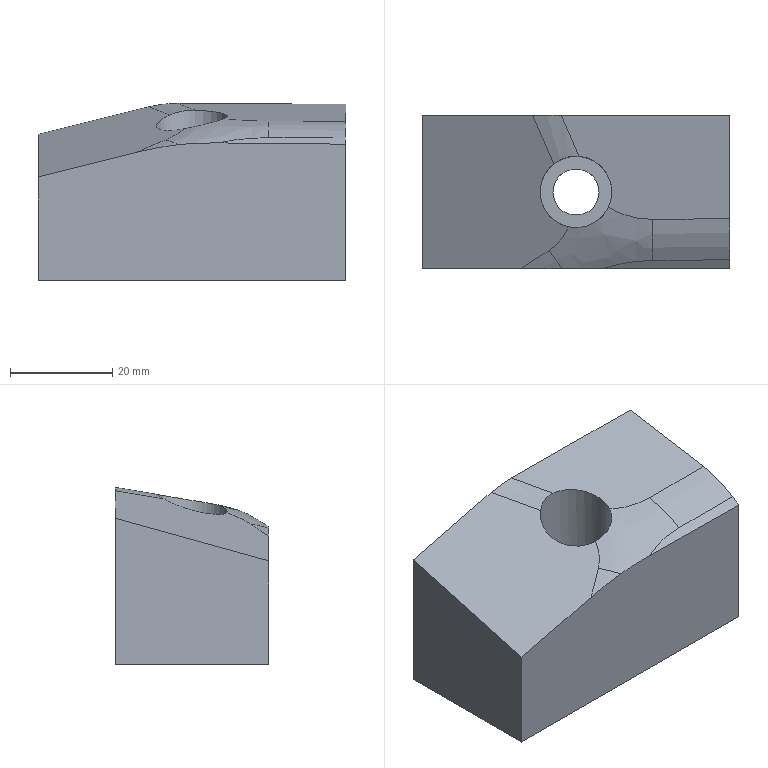Part | NX | features solid 2 | 1 solid | 15 faces | box 60 x 30.012 x 34.633 mm | volume 49926 mm3 | spline 7 | plane 6 | cylinder 2 | commonest cylinder face diameters 9 x1 14 x1
STEP:
#1=CARTESIAN_POINT('',(640.075,-255.006,46.91));
#2=VERTEX_POINT('',#1);
#3=CARTESIAN_POINT('',(665.,-255.,46.666));
#4=VERTEX_POINT('',#3);
#5=CARTESIAN_POINT('',(603.284,-255.,47.28));
#6=DIRECTION('',(1.,0.,-0.009937));
#7=VECTOR('',#6,1000.);
#8=LINE('',#5,#7);
#9=EDGE_CURVE('',#2,#4,#8,.T.);
#10=ORIENTED_EDGE('',*,*,#9,.F.);
#11=CARTESIAN_POINT('',(632.351,-255.,46.58));
#12=VERTEX_POINT('',#11);
#13=CARTESIAN_POINT('',(640.063,-255.,46.914));
#14=CARTESIAN_POINT('',(637.484,-255.,46.936));
#15=CARTESIAN_POINT('',(634.908,-255.,46.878));
#16=CARTESIAN_POINT('',(632.35,-255.,46.58));
#17=B_SPLINE_CURVE_WITH_KNOTS('',3,(#13,#14,#15,#16),.UNSPECIFIED.,.F.,.F.,(4,4),(0.007821,0.01556),.UNSPECIFIED.);
#18=EDGE_CURVE('',#2,#12,#17,.T.);
#19=ORIENTED_EDGE('',*,*,#18,.T.);
#20=CARTESIAN_POINT('',(624.182,-255.,45.074));
#21=VERTEX_POINT('',#20);
#22=CARTESIAN_POINT('',(624.182,-255.,45.074));
#23=CARTESIAN_POINT('',(626.871,-255.,45.746));
#24=CARTESIAN_POINT('',(629.597,-255.,46.262));
#25=CARTESIAN_POINT('',(632.351,-255.,46.58));
#26=B_SPLINE_CURVE_WITH_KNOTS('',3,(#22,#23,#24,#25),.UNSPECIFIED.,.F.,.F.,(4,4),(0.,0.008311),.UNSPECIFIED.);
#27=EDGE_CURVE('',#21,#12,#26,.T.);
#28=ORIENTED_EDGE('',*,*,#27,.F.);
#29=CARTESIAN_POINT('',(605.,-255.,40.28));
#30=VERTEX_POINT('',#29);
#31=CARTESIAN_POINT('',(605.,-255.,40.28));
#32=CARTESIAN_POINT('',(611.394,-255.,41.878));
#33=CARTESIAN_POINT('',(617.788,-255.,43.476));
#34=CARTESIAN_POINT('',(624.182,-255.,45.074));
#35=B_SPLINE_CURVE_WITH_KNOTS('',3,(#31,#32,#33,#34),.UNSPECIFIED.,.F.,.F.,(4,4),(0.,0.01977),.UNSPECIFIED.);
#36=EDGE_CURVE('',#30,#21,#35,.T.);
#37=ORIENTED_EDGE('',*,*,#36,.F.);
#38=CARTESIAN_POINT('',(605.,-255.,20.));
#39=VERTEX_POINT('',#38);
#40=CARTESIAN_POINT('',(605.,-255.,220.));
#41=DIRECTION('',(0.,0.,-1.));
#42=VECTOR('',#41,1000.);
#43=LINE('',#40,#42);
#44=EDGE_CURVE('',#30,#39,#43,.T.);
#45=ORIENTED_EDGE('',*,*,#44,.T.);
#46=CARTESIAN_POINT('',(665.,-255.,20.));
#47=VERTEX_POINT('',#46);
#48=CARTESIAN_POINT('',(605.,-255.,20.));
#49=DIRECTION('',(1.,0.,0.));
#50=VECTOR('',#49,1000.);
#51=LINE('',#48,#50);
#52=EDGE_CURVE('',#39,#47,#51,.T.);
#53=ORIENTED_EDGE('',*,*,#52,.T.);
#54=CARTESIAN_POINT('',(665.,-255.,220.));
#55=DIRECTION('',(0.,0.,1.));
#56=VECTOR('',#55,1000.);
#57=LINE('',#54,#56);
#58=EDGE_CURVE('',#4,#47,#57,.F.);
#59=ORIENTED_EDGE('',*,*,#58,.F.);
#60=EDGE_LOOP('',(#10,#19,#28,#37,#45,#53,#59));
#61=FACE_BOUND('',#60,.T.);
#62=CARTESIAN_POINT('',(605.,-255.,220.));
#63=DIRECTION('',(0.,1.,0.));
#64=DIRECTION('',(0.,0.,-1.));
#65=AXIS2_PLACEMENT_3D('',#62,#63,#64);
#66=PLANE('',#65);
#67=ADVANCED_FACE('',(#61),#66,.F.);
#68=CARTESIAN_POINT('',(639.5,-240.,20.));
#69=VERTEX_POINT('',#68);
#70=CARTESIAN_POINT('',(635.,-240.,20.));
#71=DIRECTION('',(0.,0.,1.));
#72=DIRECTION('',(1.,0.,0.));
#73=AXIS2_PLACEMENT_3D('',#70,#71,#72);
#74=CIRCLE('',#73,4.5);
#75=EDGE_CURVE('',#69,#69,#74,.F.);
#76=ORIENTED_EDGE('',*,*,#75,.F.);
#77=EDGE_LOOP('',(#76));
#78=FACE_BOUND('',#77,.T.);
#79=ORIENTED_EDGE('',*,*,#52,.F.);
#80=CARTESIAN_POINT('',(605.,-225.,20.));
#81=VERTEX_POINT('',#80);
#82=CARTESIAN_POINT('',(605.,-255.,20.));
#83=DIRECTION('',(0.,1.,0.));
#84=VECTOR('',#83,1000.);
#85=LINE('',#82,#84);
#86=EDGE_CURVE('',#39,#81,#85,.T.);
#87=ORIENTED_EDGE('',*,*,#86,.T.);
#88=CARTESIAN_POINT('',(665.,-225.,20.));
#89=VERTEX_POINT('',#88);
#90=CARTESIAN_POINT('',(605.,-225.,20.));
#91=DIRECTION('',(1.,0.,0.));
#92=VECTOR('',#91,1000.);
#93=LINE('',#90,#92);
#94=EDGE_CURVE('',#81,#89,#93,.T.);
#95=ORIENTED_EDGE('',*,*,#94,.T.);
#96=CARTESIAN_POINT('',(665.,-255.,20.));
#97=DIRECTION('',(0.,1.,0.));
#98=VECTOR('',#97,1000.);
#99=LINE('',#96,#98);
#100=EDGE_CURVE('',#47,#89,#99,.T.);
#101=ORIENTED_EDGE('',*,*,#100,.F.);
#102=EDGE_LOOP('',(#79,#87,#95,#101));
#103=FACE_BOUND('',#102,.T.);
#104=CARTESIAN_POINT('',(605.,-255.,20.));
#105=DIRECTION('',(0.,0.,1.));
#106=DIRECTION('',(0.,1.,0.));
#107=AXIS2_PLACEMENT_3D('',#104,#105,#106);
#108=PLANE('',#107);
#109=ADVANCED_FACE('',(#78,#103),#108,.F.);
#110=CARTESIAN_POINT('',(665.,-225.,54.456));
#111=VERTEX_POINT('',#110);
#112=CARTESIAN_POINT('',(665.,-225.,220.));
#113=DIRECTION('',(0.,0.,1.));
#114=VECTOR('',#113,1000.);
#115=LINE('',#112,#114);
#116=EDGE_CURVE('',#111,#89,#115,.F.);
#117=ORIENTED_EDGE('',*,*,#116,.F.);
#118=CARTESIAN_POINT('',(665.,-245.237,51.089));
#119=VERTEX_POINT('',#118);
#120=CARTESIAN_POINT('',(665.,-227.393,54.058));
#121=DIRECTION('',(0.,0.9864,0.1641));
#122=VECTOR('',#121,1000.);
#123=LINE('',#120,#122);
#124=EDGE_CURVE('',#111,#119,#123,.F.);
#125=ORIENTED_EDGE('',*,*,#124,.T.);
#126=CARTESIAN_POINT('',(665.,-253.26,47.859));
#127=VERTEX_POINT('',#126);
#128=CARTESIAN_POINT('',(665.,-245.237,51.089));
#129=CARTESIAN_POINT('',(665.,-248.111,50.611));
#130=CARTESIAN_POINT('',(665.,-250.857,49.505));
#131=CARTESIAN_POINT('',(665.,-253.26,47.859));
#132=B_SPLINE_CURVE_WITH_KNOTS('',3,(#128,#129,#130,#131),.UNSPECIFIED.,.F.,.F.,(4,4),(0.00005182,0.008777),.UNSPECIFIED.);
#133=EDGE_CURVE('',#119,#127,#132,.T.);
#134=ORIENTED_EDGE('',*,*,#133,.T.);
#135=CARTESIAN_POINT('',(665.,-174.178,102.045));
#136=DIRECTION('',(0.,0.8249,0.5652));
#137=VECTOR('',#136,1000.);
#138=LINE('',#135,#137);
#139=EDGE_CURVE('',#127,#4,#138,.F.);
#140=ORIENTED_EDGE('',*,*,#139,.T.);
#141=ORIENTED_EDGE('',*,*,#58,.T.);
#142=ORIENTED_EDGE('',*,*,#100,.T.);
#143=EDGE_LOOP('',(#117,#125,#134,#140,#141,#142));
#144=FACE_BOUND('',#143,.T.);
#145=CARTESIAN_POINT('',(665.,-255.,220.));
#146=DIRECTION('',(-1.,0.,0.));
#147=DIRECTION('',(0.,0.,1.));
#148=AXIS2_PLACEMENT_3D('',#145,#146,#147);
#149=PLANE('',#148);
#150=ADVANCED_FACE('',(#144),#149,.F.);
#151=CARTESIAN_POINT('',(632.136,-225.,54.632));
#152=VERTEX_POINT('',#151);
#153=CARTESIAN_POINT('',(604.112,-225.,54.783));
#154=DIRECTION('',(1.,0.,-0.005377));
#155=VECTOR('',#154,1000.);
#156=LINE('',#153,#155);
#157=EDGE_CURVE('',#111,#152,#156,.F.);
#158=ORIENTED_EDGE('',*,*,#157,.F.);
#159=ORIENTED_EDGE('',*,*,#116,.T.);
#160=ORIENTED_EDGE('',*,*,#94,.F.);
#161=CARTESIAN_POINT('',(605.,-225.,48.586));
#162=VERTEX_POINT('',#161);
#163=CARTESIAN_POINT('',(605.,-225.,220.));
#164=DIRECTION('',(0.,0.,-1.));
#165=VECTOR('',#164,1000.);
#166=LINE('',#163,#165);
#167=EDGE_CURVE('',#162,#81,#166,.T.);
#168=ORIENTED_EDGE('',*,*,#167,.F.);
#169=CARTESIAN_POINT('',(626.522,-225.,53.964));
#170=VERTEX_POINT('',#169);
#171=CARTESIAN_POINT('',(626.522,-225.,53.964));
#172=CARTESIAN_POINT('',(619.348,-225.,52.172));
#173=CARTESIAN_POINT('',(612.174,-225.,50.379));
#174=CARTESIAN_POINT('',(605.,-225.,48.586));
#175=B_SPLINE_CURVE_WITH_KNOTS('',3,(#171,#172,#173,#174),.UNSPECIFIED.,.F.,.F.,(4,4),(0.007848,0.03003),.UNSPECIFIED.);
#176=EDGE_CURVE('',#170,#162,#175,.T.);
#177=ORIENTED_EDGE('',*,*,#176,.F.);
#178=CARTESIAN_POINT('',(632.136,-225.,54.632));
#179=CARTESIAN_POINT('',(630.245,-225.,54.643));
#180=CARTESIAN_POINT('',(628.356,-225.,54.423));
#181=CARTESIAN_POINT('',(626.522,-225.,53.964));
#182=B_SPLINE_CURVE_WITH_KNOTS('',3,(#178,#179,#180,#181),.UNSPECIFIED.,.F.,.F.,(4,4),(0.,0.005662),.UNSPECIFIED.);
#183=EDGE_CURVE('',#152,#170,#182,.T.);
#184=ORIENTED_EDGE('',*,*,#183,.F.);
#185=EDGE_LOOP('',(#158,#159,#160,#168,#177,#184));
#186=FACE_BOUND('',#185,.T.);
#187=CARTESIAN_POINT('',(605.,-225.,220.));
#188=DIRECTION('',(0.,1.,0.));
#189=DIRECTION('',(0.,0.,-1.));
#190=AXIS2_PLACEMENT_3D('',#187,#188,#189);
#191=PLANE('',#190);
#192=ADVANCED_FACE('',(#186),#191,.T.);
#193=CARTESIAN_POINT('',(605.,-208.786,53.075));
#194=DIRECTION('',(0.,0.9637,0.2668));
#195=VECTOR('',#194,1000.);
#196=LINE('',#193,#195);
#197=EDGE_CURVE('',#162,#30,#196,.F.);
#198=ORIENTED_EDGE('',*,*,#197,.F.);
#199=ORIENTED_EDGE('',*,*,#167,.T.);
#200=ORIENTED_EDGE('',*,*,#86,.F.);
#201=ORIENTED_EDGE('',*,*,#44,.F.);
#202=EDGE_LOOP('',(#198,#199,#200,#201));
#203=FACE_BOUND('',#202,.T.);
#204=CARTESIAN_POINT('',(605.,-255.,220.));
#205=DIRECTION('',(-1.,0.,0.));
#206=DIRECTION('',(0.,0.,1.));
#207=AXIS2_PLACEMENT_3D('',#204,#205,#206);
#208=PLANE('',#207);
#209=ADVANCED_FACE('',(#203),#208,.T.);
#210=ORIENTED_EDGE('',*,*,#133,.F.);
#211=CARTESIAN_POINT('',(649.965,-245.37,51.148));
#212=VERTEX_POINT('',#211);
#213=CARTESIAN_POINT('',(665.,-245.237,51.089));
#214=CARTESIAN_POINT('',(659.988,-245.281,51.108));
#215=CARTESIAN_POINT('',(654.977,-245.326,51.128));
#216=CARTESIAN_POINT('',(649.965,-245.37,51.148));
#217=B_SPLINE_CURVE_WITH_KNOTS('',3,(#213,#214,#215,#216),.UNSPECIFIED.,.F.,.F.,(4,4),(0.8008,1.),.UNSPECIFIED.);
#218=EDGE_CURVE('',#212,#119,#217,.F.);
#219=ORIENTED_EDGE('',*,*,#218,.F.);
#220=CARTESIAN_POINT('',(650.023,-253.392,47.917));
#221=VERTEX_POINT('',#220);
#222=CARTESIAN_POINT('',(649.965,-245.37,51.148));
#223=CARTESIAN_POINT('',(649.988,-248.214,50.674));
#224=CARTESIAN_POINT('',(650.008,-251.014,49.546));
#225=CARTESIAN_POINT('',(650.023,-253.392,47.917));
#226=B_SPLINE_CURVE_WITH_KNOTS('',3,(#222,#223,#224,#225),.UNSPECIFIED.,.F.,.F.,(4,4),(0.,1.),.UNSPECIFIED.);
#227=EDGE_CURVE('',#212,#221,#226,.T.);
#228=ORIENTED_EDGE('',*,*,#227,.T.);
#229=CARTESIAN_POINT('',(650.023,-253.392,47.917));
#230=CARTESIAN_POINT('',(655.015,-253.348,47.898));
#231=CARTESIAN_POINT('',(660.008,-253.304,47.878));
#232=CARTESIAN_POINT('',(665.,-253.26,47.859));
#233=B_SPLINE_CURVE_WITH_KNOTS('',3,(#229,#230,#231,#232),.UNSPECIFIED.,.F.,.F.,(4,4),(0.,0.2001),.UNSPECIFIED.);
#234=EDGE_CURVE('',#221,#127,#233,.T.);
#235=ORIENTED_EDGE('',*,*,#234,.T.);
#236=EDGE_LOOP('',(#210,#219,#228,#235));
#237=FACE_BOUND('',#236,.T.);
#238=CARTESIAN_POINT('',(665.148,-253.259,47.858));
#239=CARTESIAN_POINT('',(650.023,-253.392,47.917));
#240=CARTESIAN_POINT('',(665.133,-250.843,49.514));
#241=CARTESIAN_POINT('',(650.008,-250.976,49.573));
#242=CARTESIAN_POINT('',(665.114,-248.126,50.608));
#243=CARTESIAN_POINT('',(649.988,-248.259,50.667));
#244=CARTESIAN_POINT('',(665.09,-245.237,51.088));
#245=CARTESIAN_POINT('',(649.965,-245.37,51.148));
#246=(BOUNDED_SURFACE()B_SPLINE_SURFACE(3,1,((#238,#239),(#240,#241),(#242,#243),(#244,#245)),.CYLINDRICAL_SURF.,.F.,.F.,.F.)B_SPLINE_SURFACE_WITH_KNOTS((4,4),(2,2),(0.,0.994),(0.8008,1.),.PIECEWISE_BEZIER_KNOTS.)GEOMETRIC_REPRESENTATION_ITEM()RATIONAL_B_SPLINE_SURFACE(((1.,1.),(0.9841,0.9841),(0.984,0.984),(0.9997,0.9997)))REPRESENTATION_ITEM('')SURFACE());
#247=ADVANCED_FACE('',(#237),#246,.T.);
#248=CARTESIAN_POINT('',(633.516,-246.841,49.666));
#249=VERTEX_POINT('',#248);
#250=CARTESIAN_POINT('',(629.735,-251.466,47.441));
#251=VERTEX_POINT('',#250);
#252=CARTESIAN_POINT('',(629.735,-251.466,47.44));
#253=CARTESIAN_POINT('',(630.556,-250.944,47.79));
#254=CARTESIAN_POINT('',(632.008,-249.638,48.515));
#255=CARTESIAN_POINT('',(633.064,-247.909,49.257));
#256=CARTESIAN_POINT('',(633.516,-246.841,49.666));
#257=B_SPLINE_CURVE_WITH_KNOTS('',3,(#252,#253,#254,#255,#256),.UNSPECIFIED.,.F.,.F.,(4,1,4),(0.,0.2636,0.5272),.UNSPECIFIED.);
#258=EDGE_CURVE('',#249,#251,#257,.F.);
#259=ORIENTED_EDGE('',*,*,#258,.F.);
#260=CARTESIAN_POINT('',(630.643,-234.522,52.358));
#261=VERTEX_POINT('',#260);
#262=CARTESIAN_POINT('',(633.516,-246.841,49.666));
#263=CARTESIAN_POINT('',(632.219,-246.56,49.42));
#264=CARTESIAN_POINT('',(629.723,-245.204,49.171));
#265=CARTESIAN_POINT('',(627.761,-241.464,49.716));
#266=CARTESIAN_POINT('',(628.102,-237.439,50.916));
#267=CARTESIAN_POINT('',(629.652,-235.309,51.892));
#268=CARTESIAN_POINT('',(630.643,-234.522,52.358));
#269=B_SPLINE_CURVE_WITH_KNOTS('',3,(#262,#263,#264,#265,#266,#267,#268),.UNSPECIFIED.,.F.,.F.,(4,1,1,1,4),(0.001037,0.005085,0.009132,0.01318,0.01723),.UNSPECIFIED.);
#270=EDGE_CURVE('',#249,#261,#269,.T.);
#271=ORIENTED_EDGE('',*,*,#270,.T.);
#272=CARTESIAN_POINT('',(630.643,-234.522,52.358));
#273=CARTESIAN_POINT('',(629.269,-231.348,52.894));
#274=CARTESIAN_POINT('',(627.895,-228.174,53.429));
#275=CARTESIAN_POINT('',(626.522,-225.,53.964));
#276=B_SPLINE_CURVE_WITH_KNOTS('',3,(#272,#273,#274,#275),.UNSPECIFIED.,.F.,.F.,(4,4),(0.06874,0.1608),.UNSPECIFIED.);
#277=EDGE_CURVE('',#170,#261,#276,.F.);
#278=ORIENTED_EDGE('',*,*,#277,.F.);
#279=ORIENTED_EDGE('',*,*,#176,.T.);
#280=ORIENTED_EDGE('',*,*,#197,.T.);
#281=ORIENTED_EDGE('',*,*,#36,.T.);
#282=CARTESIAN_POINT('',(624.182,-255.,45.074));
#283=CARTESIAN_POINT('',(626.033,-253.822,45.863));
#284=CARTESIAN_POINT('',(627.884,-252.644,46.652));
#285=CARTESIAN_POINT('',(629.735,-251.466,47.44));
#286=B_SPLINE_CURVE_WITH_KNOTS('',3,(#282,#283,#284,#285),.UNSPECIFIED.,.F.,.F.,(4,4),(0.868,1.),.UNSPECIFIED.);
#287=EDGE_CURVE('',#251,#21,#286,.F.);
#288=ORIENTED_EDGE('',*,*,#287,.F.);
#289=EDGE_LOOP('',(#259,#271,#278,#279,#280,#281,#288));
#290=FACE_BOUND('',#289,.T.);
#291=CARTESIAN_POINT('',(633.196,-225.095,55.606));
#292=CARTESIAN_POINT('',(633.904,-256.4,47.116));
#293=CARTESIAN_POINT('',(604.124,-223.874,48.679));
#294=CARTESIAN_POINT('',(604.832,-255.178,40.189));
#295=B_SPLINE_SURFACE_WITH_KNOTS('',1,1,((#291,#292),(#293,#294)),.PLANE_SURF.,.F.,.F.,.F.,(2,2),(2,2),(0.01963,0.6254),(0.6059,0.8264),.PIECEWISE_BEZIER_KNOTS.);
#296=ADVANCED_FACE('',(#290),#295,.T.);
#297=ORIENTED_EDGE('',*,*,#287,.T.);
#298=ORIENTED_EDGE('',*,*,#27,.T.);
#299=CARTESIAN_POINT('',(632.351,-255.,46.58));
#300=CARTESIAN_POINT('',(631.451,-253.882,47.021));
#301=CARTESIAN_POINT('',(630.569,-252.689,47.31));
#302=CARTESIAN_POINT('',(629.735,-251.466,47.44));
#303=B_SPLINE_CURVE_WITH_KNOTS('',3,(#299,#300,#301,#302),.UNSPECIFIED.,.F.,.F.,(4,4),(0.4511,1.),.UNSPECIFIED.);
#304=EDGE_CURVE('',#251,#12,#303,.F.);
#305=ORIENTED_EDGE('',*,*,#304,.F.);
#306=EDGE_LOOP('',(#297,#298,#305));
#307=FACE_BOUND('',#306,.T.);
#308=CARTESIAN_POINT('',(632.367,-255.02,46.572));
#309=CARTESIAN_POINT('',(626.78,-258.575,44.192));
#310=CARTESIAN_POINT('',(631.461,-253.896,47.018));
#311=CARTESIAN_POINT('',(625.874,-257.451,44.638));
#312=CARTESIAN_POINT('',(630.58,-252.706,47.308));
#313=CARTESIAN_POINT('',(624.993,-256.261,44.928));
#314=CARTESIAN_POINT('',(629.735,-251.466,47.44));
#315=CARTESIAN_POINT('',(624.148,-255.021,45.06));
#316=(BOUNDED_SURFACE()B_SPLINE_SURFACE(3,1,((#308,#309),(#310,#311),(#312,#313),(#314,#315)),.CYLINDRICAL_SURF.,.F.,.F.,.F.)B_SPLINE_SURFACE_WITH_KNOTS((4,4),(2,2),(0.4511,1.),(0.,0.1192),.PIECEWISE_BEZIER_KNOTS.)GEOMETRIC_REPRESENTATION_ITEM()RATIONAL_B_SPLINE_SURFACE(((0.9896,0.9896),(0.9888,0.9888),(0.9923,0.9923),(1.,1.)))REPRESENTATION_ITEM('')SURFACE());
#317=ADVANCED_FACE('',(#307),#316,.T.);
#318=ORIENTED_EDGE('',*,*,#277,.T.);
#319=CARTESIAN_POINT('',(635.61,-233.027,53.278));
#320=VERTEX_POINT('',#319);
#321=CARTESIAN_POINT('',(630.643,-234.522,52.358));
#322=CARTESIAN_POINT('',(631.98,-233.458,52.987));
#323=CARTESIAN_POINT('',(633.794,-232.868,53.314));
#324=CARTESIAN_POINT('',(635.61,-233.027,53.278));
#325=B_SPLINE_CURVE_WITH_KNOTS('',3,(#321,#322,#323,#324),.UNSPECIFIED.,.F.,.F.,(4,4),(0.,0.005439),.UNSPECIFIED.);
#326=EDGE_CURVE('',#261,#320,#325,.T.);
#327=ORIENTED_EDGE('',*,*,#326,.T.);
#328=CARTESIAN_POINT('',(635.61,-233.027,53.278));
#329=CARTESIAN_POINT('',(634.452,-230.351,53.73));
#330=CARTESIAN_POINT('',(633.294,-227.676,54.181));
#331=CARTESIAN_POINT('',(632.136,-225.,54.632));
#332=B_SPLINE_CURVE_WITH_KNOTS('',3,(#328,#329,#330,#331),.UNSPECIFIED.,.F.,.F.,(4,4),(0.06014,0.1322),.UNSPECIFIED.);
#333=EDGE_CURVE('',#152,#320,#332,.F.);
#334=ORIENTED_EDGE('',*,*,#333,.F.);
#335=ORIENTED_EDGE('',*,*,#183,.T.);
#336=EDGE_LOOP('',(#318,#327,#334,#335));
#337=FACE_BOUND('',#336,.T.);
#338=CARTESIAN_POINT('',(630.846,-234.992,52.279));
#339=CARTESIAN_POINT('',(626.496,-224.94,53.974));
#340=CARTESIAN_POINT('',(632.411,-234.408,52.832));
#341=CARTESIAN_POINT('',(628.061,-224.356,54.527));
#342=CARTESIAN_POINT('',(634.017,-233.769,53.163));
#343=CARTESIAN_POINT('',(629.667,-223.717,54.859));
#344=CARTESIAN_POINT('',(635.635,-233.086,53.268));
#345=CARTESIAN_POINT('',(631.285,-223.035,54.964));
#346=(BOUNDED_SURFACE()B_SPLINE_SURFACE(3,1,((#338,#339),(#340,#341),(#342,#343),(#344,#345)),.CYLINDRICAL_SURF.,.F.,.F.,.F.)B_SPLINE_SURFACE_WITH_KNOTS((4,4),(2,2),(0.005982,1.),(0.05925,0.1489),.PIECEWISE_BEZIER_KNOTS.)GEOMETRIC_REPRESENTATION_ITEM()RATIONAL_B_SPLINE_SURFACE(((0.9999,0.9999),(0.9942,0.9942),(0.9942,0.9942),(1.,1.)))REPRESENTATION_ITEM('')SURFACE());
#347=ADVANCED_FACE('',(#337),#346,.T.);
#348=CARTESIAN_POINT('',(641.335,-242.979,51.592));
#349=VERTEX_POINT('',#348);
#350=CARTESIAN_POINT('',(633.516,-246.841,49.666));
#351=CARTESIAN_POINT('',(635.064,-247.177,49.957));
#352=CARTESIAN_POINT('',(638.33,-246.761,50.67));
#353=CARTESIAN_POINT('',(640.659,-244.415,51.355));
#354=CARTESIAN_POINT('',(641.335,-242.979,51.592));
#355=B_SPLINE_CURVE_WITH_KNOTS('',3,(#350,#351,#352,#353,#354),.UNSPECIFIED.,.F.,.F.,(4,1,4),(0.008355,0.01314,0.01793),.UNSPECIFIED.);
#356=EDGE_CURVE('',#249,#349,#355,.T.);
#357=ORIENTED_EDGE('',*,*,#356,.F.);
#358=ORIENTED_EDGE('',*,*,#258,.T.);
#359=ORIENTED_EDGE('',*,*,#304,.T.);
#360=ORIENTED_EDGE('',*,*,#18,.F.);
#361=CARTESIAN_POINT('',(640.088,-255.012,46.906));
#362=CARTESIAN_POINT('',(640.889,-254.747,47.079));
#363=CARTESIAN_POINT('',(642.562,-254.276,47.386));
#364=CARTESIAN_POINT('',(645.818,-253.621,47.801));
#365=CARTESIAN_POINT('',(648.333,-253.407,47.924));
#366=CARTESIAN_POINT('',(650.023,-253.392,47.918));
#367=B_SPLINE_CURVE_WITH_KNOTS('',3,(#361,#362,#363,#364,#365,#366),.UNSPECIFIED.,.F.,.F.,(4,1,1,4),(0.3883,0.5412,0.6942,1.),.UNSPECIFIED.);
#368=EDGE_CURVE('',#221,#2,#367,.F.);
#369=ORIENTED_EDGE('',*,*,#368,.F.);
#370=ORIENTED_EDGE('',*,*,#227,.F.);
#371=CARTESIAN_POINT('',(649.965,-245.37,51.148));
#372=CARTESIAN_POINT('',(648.459,-245.383,51.154));
#373=CARTESIAN_POINT('',(646.227,-245.087,51.214));
#374=CARTESIAN_POINT('',(643.503,-244.18,51.381));
#375=CARTESIAN_POINT('',(641.962,-243.398,51.519));
#376=CARTESIAN_POINT('',(641.335,-242.979,51.592));
#377=B_SPLINE_CURVE_WITH_KNOTS('',3,(#371,#372,#373,#374,#375,#376),.UNSPECIFIED.,.F.,.F.,(4,1,1,4),(0.,0.3269,0.4903,0.6537),.UNSPECIFIED.);
#378=EDGE_CURVE('',#349,#212,#377,.F.);
#379=ORIENTED_EDGE('',*,*,#378,.F.);
#380=EDGE_LOOP('',(#357,#358,#359,#360,#369,#370,#379));
#381=FACE_BOUND('',#380,.T.);
#382=CARTESIAN_POINT('',(631.012,-257.176,45.293));
#383=CARTESIAN_POINT('',(630.414,-254.95,46.483));
#384=CARTESIAN_POINT('',(629.832,-252.628,47.428));
#385=CARTESIAN_POINT('',(629.287,-250.072,47.772));
#386=CARTESIAN_POINT('',(628.747,-247.484,48.036));
#387=CARTESIAN_POINT('',(628.199,-244.944,48.42));
#388=CARTESIAN_POINT('',(632.246,-256.961,45.53));
#389=CARTESIAN_POINT('',(631.645,-254.752,46.766));
#390=CARTESIAN_POINT('',(631.062,-252.437,47.728));
#391=CARTESIAN_POINT('',(630.511,-249.921,48.174));
#392=CARTESIAN_POINT('',(629.967,-247.358,48.502));
#393=CARTESIAN_POINT('',(629.417,-244.831,48.919));
#394=CARTESIAN_POINT('',(633.482,-256.737,45.744));
#395=CARTESIAN_POINT('',(632.878,-254.549,47.035));
#396=CARTESIAN_POINT('',(632.294,-252.236,48.002));
#397=CARTESIAN_POINT('',(631.736,-249.758,48.545));
#398=CARTESIAN_POINT('',(631.188,-247.221,48.939));
#399=CARTESIAN_POINT('',(630.637,-244.706,49.389));
#400=CARTESIAN_POINT('',(634.719,-256.5,45.927));
#401=CARTESIAN_POINT('',(634.111,-254.341,47.289));
#402=CARTESIAN_POINT('',(633.526,-252.036,48.278));
#403=CARTESIAN_POINT('',(632.964,-249.582,48.884));
#404=CARTESIAN_POINT('',(632.412,-247.07,49.341));
#405=CARTESIAN_POINT('',(631.858,-244.57,49.828));
#406=CARTESIAN_POINT('',(636.961,-256.059,46.224));
#407=CARTESIAN_POINT('',(636.347,-253.931,47.666));
#408=CARTESIAN_POINT('',(635.756,-251.664,48.753));
#409=CARTESIAN_POINT('',(635.19,-249.237,49.428));
#410=CARTESIAN_POINT('',(634.631,-246.771,50.004));
#411=CARTESIAN_POINT('',(634.072,-244.3,50.567));
#412=CARTESIAN_POINT('',(639.203,-255.611,46.502));
#413=CARTESIAN_POINT('',(638.587,-253.504,47.999));
#414=CARTESIAN_POINT('',(637.992,-251.254,49.129));
#415=CARTESIAN_POINT('',(637.422,-248.855,49.877));
#416=CARTESIAN_POINT('',(636.858,-246.417,50.525));
#417=CARTESIAN_POINT('',(636.299,-243.951,51.098));
#418=CARTESIAN_POINT('',(640.207,-255.41,46.626));
#419=CARTESIAN_POINT('',(639.589,-253.309,48.139));
#420=CARTESIAN_POINT('',(638.994,-251.065,49.282));
#421=CARTESIAN_POINT('',(638.421,-248.682,50.07));
#422=CARTESIAN_POINT('',(637.857,-246.243,50.716));
#423=CARTESIAN_POINT('',(637.299,-243.771,51.276));
#424=CARTESIAN_POINT('',(643.17,-254.818,46.993));
#425=CARTESIAN_POINT('',(642.55,-252.732,48.544));
#426=CARTESIAN_POINT('',(641.953,-250.5,49.721));
#427=CARTESIAN_POINT('',(641.377,-248.136,50.557));
#428=CARTESIAN_POINT('',(640.816,-245.682,51.163));
#429=CARTESIAN_POINT('',(640.261,-243.182,51.653));
#430=CARTESIAN_POINT('',(646.133,-254.227,47.364));
#431=CARTESIAN_POINT('',(645.513,-252.138,48.909));
#432=CARTESIAN_POINT('',(644.915,-249.913,50.102));
#433=CARTESIAN_POINT('',(644.343,-247.523,50.874));
#434=CARTESIAN_POINT('',(643.791,-245.014,51.338));
#435=CARTESIAN_POINT('',(643.247,-242.452,51.666));
#436=CARTESIAN_POINT('',(648.092,-253.841,47.624));
#437=CARTESIAN_POINT('',(647.473,-251.75,49.161));
#438=CARTESIAN_POINT('',(646.878,-249.502,50.297));
#439=CARTESIAN_POINT('',(646.31,-247.089,51.009));
#440=CARTESIAN_POINT('',(645.763,-244.548,51.392));
#441=CARTESIAN_POINT('',(645.224,-241.956,51.642));
#442=CARTESIAN_POINT('',(650.051,-253.456,47.885));
#443=CARTESIAN_POINT('',(649.436,-251.338,49.353));
#444=CARTESIAN_POINT('',(648.846,-249.065,50.425));
#445=CARTESIAN_POINT('',(648.277,-246.657,51.147));
#446=CARTESIAN_POINT('',(647.735,-244.083,51.446));
#447=CARTESIAN_POINT('',(647.202,-241.451,51.594));
#448=CARTESIAN_POINT('',(652.012,-253.06,48.117));
#449=CARTESIAN_POINT('',(651.401,-250.915,49.517));
#450=CARTESIAN_POINT('',(650.812,-248.635,50.568));
#451=CARTESIAN_POINT('',(650.246,-246.213,51.257));
#452=CARTESIAN_POINT('',(649.709,-243.604,51.466));
#453=CARTESIAN_POINT('',(649.182,-240.934,51.518));
#454=B_SPLINE_SURFACE_WITH_KNOTS('',5,5,((#382,#383,#384,#385,#386,#387),(#388,#389,#390,#391,#392,#393),(#394,#395,#396,#397,#398,#399),(#400,#401,#402,#403,#404,#405),(#406,#407,#408,#409,#410,#411),(#412,#413,#414,#415,#416,#417),(#418,#419,#420,#421,#422,#423),(#424,#425,#426,#427,#428,#429),(#430,#431,#432,#433,#434,#435),(#436,#437,#438,#439,#440,#441),(#442,#443,#444,#445,#446,#447),(#448,#449,#450,#451,#452,#453)),.UNSPECIFIED.,.F.,.F.,.F.,(6,3,3,6),(6,6),(0.,0.2949,0.5336,1.),(0.07289,0.7877),.UNSPECIFIED.);
#455=ADVANCED_FACE('',(#381),#454,.T.);
#456=ORIENTED_EDGE('',*,*,#368,.T.);
#457=ORIENTED_EDGE('',*,*,#9,.T.);
#458=ORIENTED_EDGE('',*,*,#139,.F.);
#459=ORIENTED_EDGE('',*,*,#234,.F.);
#460=EDGE_LOOP('',(#456,#457,#458,#459));
#461=FACE_BOUND('',#460,.T.);
#462=CARTESIAN_POINT('',(639.939,-253.366,48.035));
#463=CARTESIAN_POINT('',(665.,-253.25,47.866));
#464=CARTESIAN_POINT('',(639.939,-255.127,46.829));
#465=CARTESIAN_POINT('',(665.,-255.01,46.659));
#466=B_SPLINE_SURFACE_WITH_KNOTS('',1,1,((#462,#463),(#464,#465)),.PLANE_SURF.,.F.,.F.,.F.,(2,2),(2,2),(0.01244,0.06058),(0.3856,0.5651),.PIECEWISE_BEZIER_KNOTS.);
#467=ADVANCED_FACE('',(#461),#466,.T.);
#468=ORIENTED_EDGE('',*,*,#333,.T.);
#469=CARTESIAN_POINT('',(635.61,-233.027,53.278));
#470=CARTESIAN_POINT('',(637.855,-233.223,53.234));
#471=CARTESIAN_POINT('',(642.093,-235.975,52.753));
#472=CARTESIAN_POINT('',(642.284,-240.96,51.923));
#473=CARTESIAN_POINT('',(641.335,-242.979,51.592));
#474=B_SPLINE_CURVE_WITH_KNOTS('',3,(#469,#470,#471,#472,#473),.UNSPECIFIED.,.F.,.F.,(4,1,4),(0.003765,0.01052,0.01728),.UNSPECIFIED.);
#475=EDGE_CURVE('',#320,#349,#474,.T.);
#476=ORIENTED_EDGE('',*,*,#475,.T.);
#477=ORIENTED_EDGE('',*,*,#378,.T.);
#478=ORIENTED_EDGE('',*,*,#218,.T.);
#479=ORIENTED_EDGE('',*,*,#124,.F.);
#480=ORIENTED_EDGE('',*,*,#157,.T.);
#481=EDGE_LOOP('',(#468,#476,#477,#478,#479,#480));
#482=FACE_BOUND('',#481,.T.);
#483=CARTESIAN_POINT('',(631.939,-224.878,54.654));
#484=CARTESIAN_POINT('',(665.,-224.849,54.481));
#485=CARTESIAN_POINT('',(631.939,-245.535,51.217));
#486=CARTESIAN_POINT('',(665.,-245.506,51.044));
#487=B_SPLINE_SURFACE_WITH_KNOTS('',1,1,((#483,#484),(#485,#486)),.PLANE_SURF.,.F.,.F.,.F.,(2,2),(2,2),(0.8446,0.9951),(0.3209,0.5589),.PIECEWISE_BEZIER_KNOTS.);
#488=ADVANCED_FACE('',(#482),#487,.T.);
#489=CARTESIAN_POINT('',(642.,-240.,30.));
#490=VERTEX_POINT('',#489);
#491=CARTESIAN_POINT('',(635.,-240.,30.));
#492=DIRECTION('',(0.,0.,1.));
#493=DIRECTION('',(1.,0.,0.));
#494=AXIS2_PLACEMENT_3D('',#491,#492,#493);
#495=CIRCLE('',#494,7.);
#496=EDGE_CURVE('',#490,#490,#495,.T.);
#497=ORIENTED_EDGE('',*,*,#496,.F.);
#498=EDGE_LOOP('',(#497));
#499=FACE_BOUND('',#498,.T.);
#500=ORIENTED_EDGE('',*,*,#326,.F.);
#501=ORIENTED_EDGE('',*,*,#270,.F.);
#502=ORIENTED_EDGE('',*,*,#356,.T.);
#503=ORIENTED_EDGE('',*,*,#475,.F.);
#504=EDGE_LOOP('',(#500,#501,#502,#503));
#505=FACE_BOUND('',#504,.T.);
#506=CARTESIAN_POINT('',(635.,-240.,30.));
#507=DIRECTION('',(0.,0.,1.));
#508=DIRECTION('',(1.,0.,0.));
#509=AXIS2_PLACEMENT_3D('',#506,#507,#508);
#510=CYLINDRICAL_SURFACE('',#509,7.);
#511=ADVANCED_FACE('',(#499,#505),#510,.F.);
#512=CARTESIAN_POINT('',(630.5,-240.,30.));
#513=VERTEX_POINT('',#512);
#514=CARTESIAN_POINT('',(635.,-240.,30.));
#515=DIRECTION('',(0.,0.,-1.));
#516=DIRECTION('',(-1.,0.,0.));
#517=AXIS2_PLACEMENT_3D('',#514,#515,#516);
#518=CIRCLE('',#517,4.5);
#519=EDGE_CURVE('',#513,#513,#518,.T.);
#520=ORIENTED_EDGE('',*,*,#519,.T.);
#521=EDGE_LOOP('',(#520));
#522=FACE_BOUND('',#521,.T.);
#523=ORIENTED_EDGE('',*,*,#496,.T.);
#524=EDGE_LOOP('',(#523));
#525=FACE_BOUND('',#524,.T.);
#526=CARTESIAN_POINT('',(635.,-240.,30.));
#527=DIRECTION('',(0.,0.,-1.));
#528=DIRECTION('',(-1.,0.,0.));
#529=AXIS2_PLACEMENT_3D('',#526,#527,#528);
#530=PLANE('',#529);
#531=ADVANCED_FACE('',(#522,#525),#530,.F.);
#532=ORIENTED_EDGE('',*,*,#75,.T.);
#533=EDGE_LOOP('',(#532));
#534=FACE_BOUND('',#533,.T.);
#535=ORIENTED_EDGE('',*,*,#519,.F.);
#536=EDGE_LOOP('',(#535));
#537=FACE_BOUND('',#536,.T.);
#538=CARTESIAN_POINT('',(635.,-240.,30.));
#539=DIRECTION('',(0.,0.,-1.));
#540=DIRECTION('',(-1.,0.,0.));
#541=AXIS2_PLACEMENT_3D('',#538,#539,#540);
#542=CYLINDRICAL_SURFACE('',#541,4.5);
#543=ADVANCED_FACE('',(#534,#537),#542,.F.);
#544=CLOSED_SHELL('',(#67,#109,#150,#192,#209,#247,#296,#317,#347,#455,#467,#488,#511,#531,#543));
#545=MANIFOLD_SOLID_BREP('',#544);
#546=(LENGTH_UNIT()NAMED_UNIT(*)SI_UNIT(.MILLI.,.METRE.));
#547=UNCERTAINTY_MEASURE_WITH_UNIT(LENGTH_MEASURE(0.1584),#546,'','');
#548=(NAMED_UNIT(*)PLANE_ANGLE_UNIT()SI_UNIT($,.RADIAN.));
#549=(NAMED_UNIT(*)SI_UNIT($,.STERADIAN.)SOLID_ANGLE_UNIT());
#550=(GEOMETRIC_REPRESENTATION_CONTEXT(3)GLOBAL_UNCERTAINTY_ASSIGNED_CONTEXT((#547))GLOBAL_UNIT_ASSIGNED_CONTEXT((#546,#548,#549))REPRESENTATION_CONTEXT('',''));
#551=ADVANCED_BREP_SHAPE_REPRESENTATION('',(#545),#550);